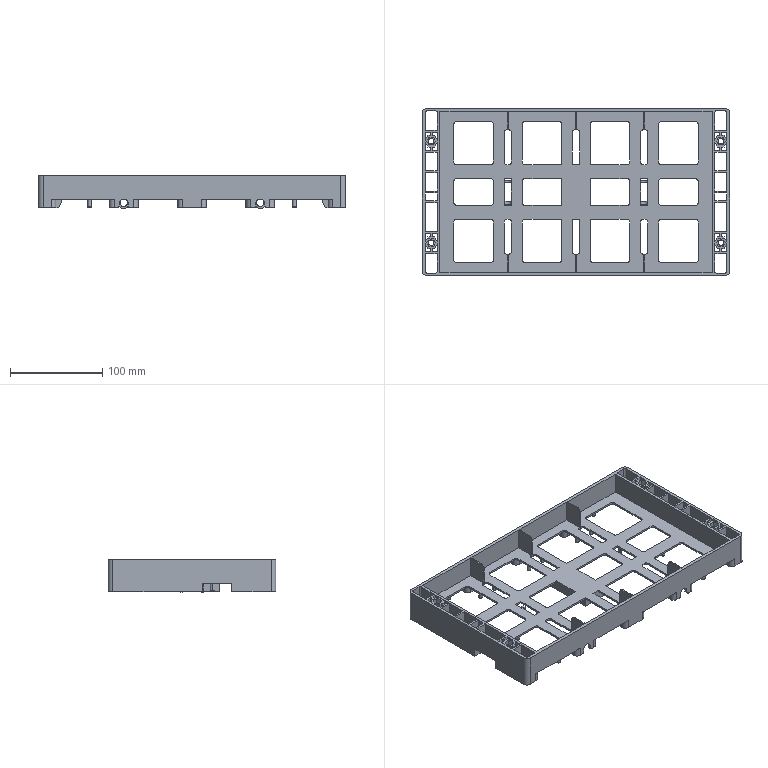Part | NX | features BREP 1 | 1 solid | 756 faces | box 333 x 182 x 35.5 mm | volume 236706 mm3 | plane 498 | cylinder 206 | cone 48 | torus 4 | commonest cylinder face diameters 4 x84 6 x68 10 x46 8 x4 12 x4